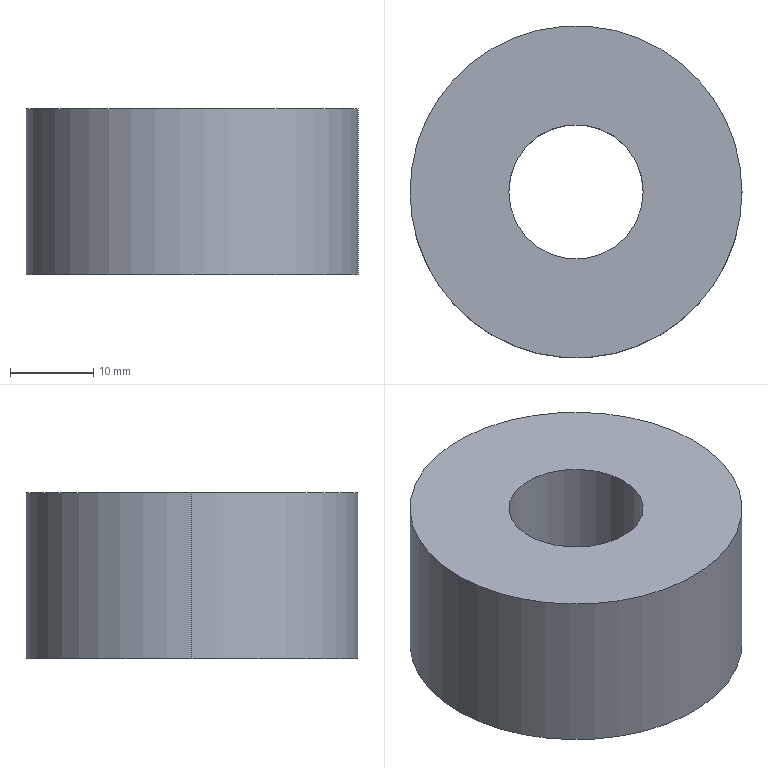Part | SolidWorks | features Extrusion 1 | 1 solid | 6 faces | box 40 x 40 x 20 mm | volume 21010 mm3 | cylinder 4 | plane 2 | commonest cylinder face diameters 16.2 x2 40 x2
STEP:
#1=CARTESIAN_POINT('',(-8.1,0.,-10.));
#2=VERTEX_POINT('',#1);
#3=CARTESIAN_POINT('',(8.1,0.,-10.));
#4=VERTEX_POINT('',#3);
#5=CARTESIAN_POINT('',(0.,0.,-10.));
#6=DIRECTION('',(0.,0.,1.));
#7=DIRECTION('',(1.,0.,0.));
#8=AXIS2_PLACEMENT_3D('',#5,#6,#7);
#9=CIRCLE('',#8,8.1);
#10=EDGE_CURVE('',#2,#4,#9,.T.);
#11=ORIENTED_EDGE('',*,*,#10,.F.);
#12=CARTESIAN_POINT('',(-8.1,0.,10.));
#13=VERTEX_POINT('',#12);
#14=CARTESIAN_POINT('',(-8.1,0.,-10.));
#15=DIRECTION('',(0.,0.,1.));
#16=VECTOR('',#15,1000.);
#17=LINE('',#14,#16);
#18=EDGE_CURVE('',#2,#13,#17,.T.);
#19=ORIENTED_EDGE('',*,*,#18,.T.);
#20=CARTESIAN_POINT('',(8.1,0.,10.));
#21=VERTEX_POINT('',#20);
#22=CARTESIAN_POINT('',(0.,0.,10.));
#23=DIRECTION('',(0.,0.,1.));
#24=DIRECTION('',(1.,0.,0.));
#25=AXIS2_PLACEMENT_3D('',#22,#23,#24);
#26=CIRCLE('',#25,8.1);
#27=EDGE_CURVE('',#13,#21,#26,.T.);
#28=ORIENTED_EDGE('',*,*,#27,.T.);
#29=CARTESIAN_POINT('',(8.1,0.,-10.));
#30=DIRECTION('',(0.,0.,1.));
#31=VECTOR('',#30,1000.);
#32=LINE('',#29,#31);
#33=EDGE_CURVE('',#4,#21,#32,.T.);
#34=ORIENTED_EDGE('',*,*,#33,.F.);
#35=EDGE_LOOP('',(#11,#19,#28,#34));
#36=FACE_OUTER_BOUND('',#35,.T.);
#37=CARTESIAN_POINT('',(0.,0.,-10.));
#38=DIRECTION('',(0.,0.,1.));
#39=DIRECTION('',(1.,0.,0.));
#40=AXIS2_PLACEMENT_3D('',#37,#38,#39);
#41=CYLINDRICAL_SURFACE('',#40,8.1);
#42=ADVANCED_FACE('',(#36),#41,.F.);
#43=CARTESIAN_POINT('',(20.,0.,-10.));
#44=VERTEX_POINT('',#43);
#45=CARTESIAN_POINT('',(-20.,0.,-10.));
#46=VERTEX_POINT('',#45);
#47=CARTESIAN_POINT('',(0.,0.,-10.));
#48=DIRECTION('',(0.,0.,1.));
#49=DIRECTION('',(1.,0.,0.));
#50=AXIS2_PLACEMENT_3D('',#47,#48,#49);
#51=CIRCLE('',#50,20.);
#52=EDGE_CURVE('',#44,#46,#51,.T.);
#53=ORIENTED_EDGE('',*,*,#52,.T.);
#54=CARTESIAN_POINT('',(-20.,0.,10.));
#55=VERTEX_POINT('',#54);
#56=CARTESIAN_POINT('',(-20.,0.,-10.));
#57=DIRECTION('',(0.,0.,1.));
#58=VECTOR('',#57,1000.);
#59=LINE('',#56,#58);
#60=EDGE_CURVE('',#46,#55,#59,.T.);
#61=ORIENTED_EDGE('',*,*,#60,.T.);
#62=CARTESIAN_POINT('',(20.,0.,10.));
#63=VERTEX_POINT('',#62);
#64=CARTESIAN_POINT('',(0.,0.,10.));
#65=DIRECTION('',(0.,0.,1.));
#66=DIRECTION('',(1.,0.,0.));
#67=AXIS2_PLACEMENT_3D('',#64,#65,#66);
#68=CIRCLE('',#67,20.);
#69=EDGE_CURVE('',#63,#55,#68,.T.);
#70=ORIENTED_EDGE('',*,*,#69,.F.);
#71=CARTESIAN_POINT('',(20.,0.,-10.));
#72=DIRECTION('',(0.,0.,1.));
#73=VECTOR('',#72,1000.);
#74=LINE('',#71,#73);
#75=EDGE_CURVE('',#44,#63,#74,.T.);
#76=ORIENTED_EDGE('',*,*,#75,.F.);
#77=EDGE_LOOP('',(#53,#61,#70,#76));
#78=FACE_OUTER_BOUND('',#77,.T.);
#79=CARTESIAN_POINT('',(0.,0.,-10.));
#80=DIRECTION('',(0.,0.,1.));
#81=DIRECTION('',(1.,0.,0.));
#82=AXIS2_PLACEMENT_3D('',#79,#80,#81);
#83=CYLINDRICAL_SURFACE('',#82,20.);
#84=ADVANCED_FACE('',(#78),#83,.T.);
#85=ORIENTED_EDGE('',*,*,#60,.F.);
#86=CARTESIAN_POINT('',(0.,0.,-10.));
#87=DIRECTION('',(0.,0.,1.));
#88=DIRECTION('',(1.,0.,0.));
#89=AXIS2_PLACEMENT_3D('',#86,#87,#88);
#90=CIRCLE('',#89,20.);
#91=EDGE_CURVE('',#46,#44,#90,.T.);
#92=ORIENTED_EDGE('',*,*,#91,.T.);
#93=ORIENTED_EDGE('',*,*,#75,.T.);
#94=CARTESIAN_POINT('',(0.,0.,10.));
#95=DIRECTION('',(0.,0.,1.));
#96=DIRECTION('',(1.,0.,0.));
#97=AXIS2_PLACEMENT_3D('',#94,#95,#96);
#98=CIRCLE('',#97,20.);
#99=EDGE_CURVE('',#55,#63,#98,.T.);
#100=ORIENTED_EDGE('',*,*,#99,.F.);
#101=EDGE_LOOP('',(#85,#92,#93,#100));
#102=FACE_OUTER_BOUND('',#101,.T.);
#103=CARTESIAN_POINT('',(0.,0.,-10.));
#104=DIRECTION('',(0.,0.,1.));
#105=DIRECTION('',(1.,0.,0.));
#106=AXIS2_PLACEMENT_3D('',#103,#104,#105);
#107=CYLINDRICAL_SURFACE('',#106,20.);
#108=ADVANCED_FACE('',(#102),#107,.T.);
#109=CARTESIAN_POINT('',(0.,0.,-10.));
#110=DIRECTION('',(0.,0.,1.));
#111=DIRECTION('',(1.,0.,0.));
#112=AXIS2_PLACEMENT_3D('',#109,#110,#111);
#113=CIRCLE('',#112,8.1);
#114=EDGE_CURVE('',#4,#2,#113,.T.);
#115=ORIENTED_EDGE('',*,*,#114,.T.);
#116=ORIENTED_EDGE('',*,*,#10,.T.);
#117=EDGE_LOOP('',(#115,#116));
#118=FACE_BOUND('',#117,.T.);
#119=ORIENTED_EDGE('',*,*,#52,.F.);
#120=ORIENTED_EDGE('',*,*,#91,.F.);
#121=EDGE_LOOP('',(#119,#120));
#122=FACE_OUTER_BOUND('',#121,.T.);
#123=CARTESIAN_POINT('',(0.,0.,-10.));
#124=DIRECTION('',(0.,0.,1.));
#125=DIRECTION('',(1.,0.,0.));
#126=AXIS2_PLACEMENT_3D('',#123,#124,#125);
#127=PLANE('',#126);
#128=ADVANCED_FACE('',(#118,#122),#127,.F.);
#129=CARTESIAN_POINT('',(0.,0.,10.));
#130=DIRECTION('',(0.,0.,1.));
#131=DIRECTION('',(1.,0.,0.));
#132=AXIS2_PLACEMENT_3D('',#129,#130,#131);
#133=CIRCLE('',#132,8.1);
#134=EDGE_CURVE('',#21,#13,#133,.T.);
#135=ORIENTED_EDGE('',*,*,#134,.F.);
#136=ORIENTED_EDGE('',*,*,#27,.F.);
#137=EDGE_LOOP('',(#135,#136));
#138=FACE_BOUND('',#137,.T.);
#139=ORIENTED_EDGE('',*,*,#69,.T.);
#140=ORIENTED_EDGE('',*,*,#99,.T.);
#141=EDGE_LOOP('',(#139,#140));
#142=FACE_OUTER_BOUND('',#141,.T.);
#143=CARTESIAN_POINT('',(0.,0.,10.));
#144=DIRECTION('',(0.,0.,1.));
#145=DIRECTION('',(1.,0.,0.));
#146=AXIS2_PLACEMENT_3D('',#143,#144,#145);
#147=PLANE('',#146);
#148=ADVANCED_FACE('',(#138,#142),#147,.T.);
#149=ORIENTED_EDGE('',*,*,#18,.F.);
#150=ORIENTED_EDGE('',*,*,#114,.F.);
#151=ORIENTED_EDGE('',*,*,#33,.T.);
#152=ORIENTED_EDGE('',*,*,#134,.T.);
#153=EDGE_LOOP('',(#149,#150,#151,#152));
#154=FACE_OUTER_BOUND('',#153,.T.);
#155=CARTESIAN_POINT('',(0.,0.,-10.));
#156=DIRECTION('',(0.,0.,1.));
#157=DIRECTION('',(1.,0.,0.));
#158=AXIS2_PLACEMENT_3D('',#155,#156,#157);
#159=CYLINDRICAL_SURFACE('',#158,8.1);
#160=ADVANCED_FACE('',(#154),#159,.F.);
#161=CLOSED_SHELL('',(#42,#84,#108,#128,#148,#160));
#162=MANIFOLD_SOLID_BREP('',#161);
#163=CARTESIAN_POINT('',(0.,0.,0.));
#164=DIRECTION('',(0.,0.,1.));
#165=DIRECTION('',(1.,0.,0.));
#166=AXIS2_PLACEMENT_3D('',#163,#164,#165);
#167=(LENGTH_UNIT()NAMED_UNIT(*)SI_UNIT(.MILLI.,.METRE.));
#168=UNCERTAINTY_MEASURE_WITH_UNIT(LENGTH_MEASURE(0.00001),#167,'','');
#169=(NAMED_UNIT(*)PLANE_ANGLE_UNIT()SI_UNIT($,.RADIAN.));
#170=(NAMED_UNIT(*)SI_UNIT($,.STERADIAN.)SOLID_ANGLE_UNIT());
#171=(GEOMETRIC_REPRESENTATION_CONTEXT(3)GLOBAL_UNCERTAINTY_ASSIGNED_CONTEXT((#168))GLOBAL_UNIT_ASSIGNED_CONTEXT((#167,#169,#170))REPRESENTATION_CONTEXT('',''));
#172=ADVANCED_BREP_SHAPE_REPRESENTATION('',(#162,#166),#171);